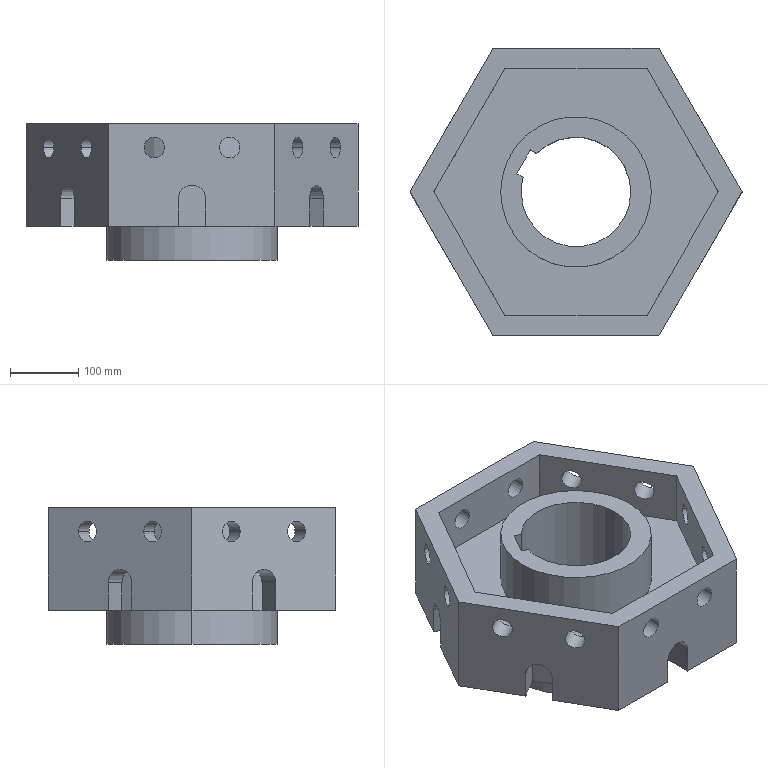Part | NX | features BREP 1 | 1 solid | 78 faces | box 484.974 x 420 x 200 mm | volume 14525982 mm3 | cylinder 39 | plane 39 | commonest cylinder face diameters 30 x24 40 x6 160 x3 14 x2 220 x2 250 x2